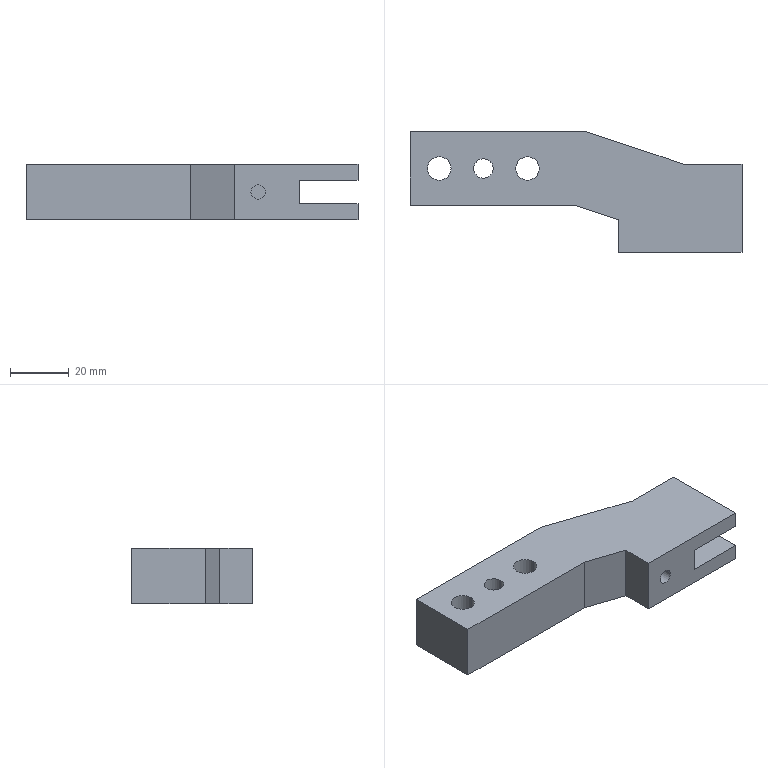Part | SolidWorks | features ICE 2, Extrusion 1 | 1 solid | 25 faces | box 113 x 41 x 19 mm | volume 51873 mm3 | plane 17 | cylinder 8 | commonest cylinder face diameters 8 x4 4.917 x2 6.647 x2
STEP:
#1=CARTESIAN_POINT('',(76.542,-1.,9.5));
#2=VERTEX_POINT('',#1);
#3=CARTESIAN_POINT('',(81.459,-1.,9.5));
#4=VERTEX_POINT('',#3);
#5=CARTESIAN_POINT('',(79.,-1.,9.5));
#6=DIRECTION('',(0.,-1.,0.));
#7=DIRECTION('',(1.,0.,0.));
#8=AXIS2_PLACEMENT_3D('',#5,#6,#7);
#9=CIRCLE('',#8,2.459);
#10=EDGE_CURVE('',#2,#4,#9,.T.);
#11=ORIENTED_EDGE('',*,*,#10,.F.);
#12=CARTESIAN_POINT('',(76.542,-16.,9.5));
#13=VERTEX_POINT('',#12);
#14=CARTESIAN_POINT('',(76.542,-1.,9.5));
#15=DIRECTION('',(0.,-1.,0.));
#16=VECTOR('',#15,1000.);
#17=LINE('',#14,#16);
#18=EDGE_CURVE('',#2,#13,#17,.T.);
#19=ORIENTED_EDGE('',*,*,#18,.T.);
#20=CARTESIAN_POINT('',(81.459,-16.,9.5));
#21=VERTEX_POINT('',#20);
#22=CARTESIAN_POINT('',(79.,-16.,9.5));
#23=DIRECTION('',(0.,-1.,0.));
#24=DIRECTION('',(1.,0.,0.));
#25=AXIS2_PLACEMENT_3D('',#22,#23,#24);
#26=CIRCLE('',#25,2.459);
#27=EDGE_CURVE('',#13,#21,#26,.T.);
#28=ORIENTED_EDGE('',*,*,#27,.T.);
#29=CARTESIAN_POINT('',(81.459,-1.,9.5));
#30=DIRECTION('',(0.,-1.,0.));
#31=VECTOR('',#30,1000.);
#32=LINE('',#29,#31);
#33=EDGE_CURVE('',#4,#21,#32,.T.);
#34=ORIENTED_EDGE('',*,*,#33,.F.);
#35=EDGE_LOOP('',(#11,#19,#28,#34));
#36=FACE_OUTER_BOUND('',#35,.T.);
#37=CARTESIAN_POINT('',(79.,-1.,9.5));
#38=DIRECTION('',(0.,-1.,0.));
#39=DIRECTION('',(1.,0.,0.));
#40=AXIS2_PLACEMENT_3D('',#37,#38,#39);
#41=CYLINDRICAL_SURFACE('',#40,2.459);
#42=ADVANCED_FACE('',(#36),#41,.F.);
#43=CARTESIAN_POINT('',(36.,12.5,19.));
#44=VERTEX_POINT('',#43);
#45=CARTESIAN_POINT('',(44.,12.5,19.));
#46=VERTEX_POINT('',#45);
#47=CARTESIAN_POINT('',(40.,12.5,19.));
#48=DIRECTION('',(0.,0.,1.));
#49=DIRECTION('',(1.,0.,0.));
#50=AXIS2_PLACEMENT_3D('',#47,#48,#49);
#51=CIRCLE('',#50,4.);
#52=EDGE_CURVE('',#44,#46,#51,.T.);
#53=ORIENTED_EDGE('',*,*,#52,.T.);
#54=CARTESIAN_POINT('',(44.,12.5,0.));
#55=VERTEX_POINT('',#54);
#56=CARTESIAN_POINT('',(44.,12.5,19.));
#57=DIRECTION('',(0.,0.,-1.));
#58=VECTOR('',#57,1000.);
#59=LINE('',#56,#58);
#60=EDGE_CURVE('',#46,#55,#59,.T.);
#61=ORIENTED_EDGE('',*,*,#60,.T.);
#62=CARTESIAN_POINT('',(36.,12.5,0.));
#63=VERTEX_POINT('',#62);
#64=CARTESIAN_POINT('',(40.,12.5,0.));
#65=DIRECTION('',(0.,0.,1.));
#66=DIRECTION('',(1.,0.,0.));
#67=AXIS2_PLACEMENT_3D('',#64,#65,#66);
#68=CIRCLE('',#67,4.);
#69=EDGE_CURVE('',#63,#55,#68,.T.);
#70=ORIENTED_EDGE('',*,*,#69,.F.);
#71=CARTESIAN_POINT('',(36.,12.5,19.));
#72=DIRECTION('',(0.,0.,-1.));
#73=VECTOR('',#72,1000.);
#74=LINE('',#71,#73);
#75=EDGE_CURVE('',#44,#63,#74,.T.);
#76=ORIENTED_EDGE('',*,*,#75,.F.);
#77=EDGE_LOOP('',(#53,#61,#70,#76));
#78=FACE_OUTER_BOUND('',#77,.T.);
#79=CARTESIAN_POINT('',(40.,12.5,19.));
#80=DIRECTION('',(0.,0.,-1.));
#81=DIRECTION('',(-1.,0.,0.));
#82=AXIS2_PLACEMENT_3D('',#79,#80,#81);
#83=CYLINDRICAL_SURFACE('',#82,4.);
#84=ADVANCED_FACE('',(#78),#83,.F.);
#85=CARTESIAN_POINT('',(21.677,12.5,19.));
#86=VERTEX_POINT('',#85);
#87=CARTESIAN_POINT('',(28.324,12.5,19.));
#88=VERTEX_POINT('',#87);
#89=CARTESIAN_POINT('',(25.,12.5,19.));
#90=DIRECTION('',(0.,0.,1.));
#91=DIRECTION('',(1.,0.,0.));
#92=AXIS2_PLACEMENT_3D('',#89,#90,#91);
#93=CIRCLE('',#92,3.324);
#94=EDGE_CURVE('',#86,#88,#93,.T.);
#95=ORIENTED_EDGE('',*,*,#94,.T.);
#96=CARTESIAN_POINT('',(28.324,12.5,0.));
#97=VERTEX_POINT('',#96);
#98=CARTESIAN_POINT('',(28.324,12.5,19.));
#99=DIRECTION('',(0.,0.,-1.));
#100=VECTOR('',#99,1000.);
#101=LINE('',#98,#100);
#102=EDGE_CURVE('',#88,#97,#101,.T.);
#103=ORIENTED_EDGE('',*,*,#102,.T.);
#104=CARTESIAN_POINT('',(21.677,12.5,0.));
#105=VERTEX_POINT('',#104);
#106=CARTESIAN_POINT('',(25.,12.5,0.));
#107=DIRECTION('',(0.,0.,1.));
#108=DIRECTION('',(1.,0.,0.));
#109=AXIS2_PLACEMENT_3D('',#106,#107,#108);
#110=CIRCLE('',#109,3.324);
#111=EDGE_CURVE('',#105,#97,#110,.T.);
#112=ORIENTED_EDGE('',*,*,#111,.F.);
#113=CARTESIAN_POINT('',(21.677,12.5,19.));
#114=DIRECTION('',(0.,0.,-1.));
#115=VECTOR('',#114,1000.);
#116=LINE('',#113,#115);
#117=EDGE_CURVE('',#86,#105,#116,.T.);
#118=ORIENTED_EDGE('',*,*,#117,.F.);
#119=EDGE_LOOP('',(#95,#103,#112,#118));
#120=FACE_OUTER_BOUND('',#119,.T.);
#121=CARTESIAN_POINT('',(25.,12.5,19.));
#122=DIRECTION('',(0.,0.,-1.));
#123=DIRECTION('',(-1.,0.,0.));
#124=AXIS2_PLACEMENT_3D('',#121,#122,#123);
#125=CYLINDRICAL_SURFACE('',#124,3.324);
#126=ADVANCED_FACE('',(#120),#125,.F.);
#127=CARTESIAN_POINT('',(6.,12.5,19.));
#128=VERTEX_POINT('',#127);
#129=CARTESIAN_POINT('',(14.,12.5,19.));
#130=VERTEX_POINT('',#129);
#131=CARTESIAN_POINT('',(10.,12.5,19.));
#132=DIRECTION('',(0.,0.,1.));
#133=DIRECTION('',(1.,0.,0.));
#134=AXIS2_PLACEMENT_3D('',#131,#132,#133);
#135=CIRCLE('',#134,4.);
#136=EDGE_CURVE('',#128,#130,#135,.T.);
#137=ORIENTED_EDGE('',*,*,#136,.T.);
#138=CARTESIAN_POINT('',(14.,12.5,0.));
#139=VERTEX_POINT('',#138);
#140=CARTESIAN_POINT('',(14.,12.5,19.));
#141=DIRECTION('',(0.,0.,-1.));
#142=VECTOR('',#141,1000.);
#143=LINE('',#140,#142);
#144=EDGE_CURVE('',#130,#139,#143,.T.);
#145=ORIENTED_EDGE('',*,*,#144,.T.);
#146=CARTESIAN_POINT('',(6.,12.5,0.));
#147=VERTEX_POINT('',#146);
#148=CARTESIAN_POINT('',(10.,12.5,0.));
#149=DIRECTION('',(0.,0.,1.));
#150=DIRECTION('',(1.,0.,0.));
#151=AXIS2_PLACEMENT_3D('',#148,#149,#150);
#152=CIRCLE('',#151,4.);
#153=EDGE_CURVE('',#147,#139,#152,.T.);
#154=ORIENTED_EDGE('',*,*,#153,.F.);
#155=CARTESIAN_POINT('',(6.,12.5,19.));
#156=DIRECTION('',(0.,0.,-1.));
#157=VECTOR('',#156,1000.);
#158=LINE('',#155,#157);
#159=EDGE_CURVE('',#128,#147,#158,.T.);
#160=ORIENTED_EDGE('',*,*,#159,.F.);
#161=EDGE_LOOP('',(#137,#145,#154,#160));
#162=FACE_OUTER_BOUND('',#161,.T.);
#163=CARTESIAN_POINT('',(10.,12.5,19.));
#164=DIRECTION('',(0.,0.,-1.));
#165=DIRECTION('',(-1.,0.,0.));
#166=AXIS2_PLACEMENT_3D('',#163,#164,#165);
#167=CYLINDRICAL_SURFACE('',#166,4.);
#168=ADVANCED_FACE('',(#162),#167,.F.);
#169=CARTESIAN_POINT('',(113.,14.,5.5));
#170=VERTEX_POINT('',#169);
#171=CARTESIAN_POINT('',(113.,14.,0.));
#172=VERTEX_POINT('',#171);
#173=CARTESIAN_POINT('',(113.,14.,19.));
#174=DIRECTION('',(0.,0.,-1.));
#175=VECTOR('',#174,1000.);
#176=LINE('',#173,#175);
#177=EDGE_CURVE('',#170,#172,#176,.T.);
#178=ORIENTED_EDGE('',*,*,#177,.F.);
#179=CARTESIAN_POINT('',(113.,-16.,5.5));
#180=VERTEX_POINT('',#179);
#181=CARTESIAN_POINT('',(113.,-16.001,5.5));
#182=DIRECTION('',(0.,1.,0.));
#183=VECTOR('',#182,1000.);
#184=LINE('',#181,#183);
#185=EDGE_CURVE('',#180,#170,#184,.T.);
#186=ORIENTED_EDGE('',*,*,#185,.F.);
#187=CARTESIAN_POINT('',(113.,-16.,0.));
#188=VERTEX_POINT('',#187);
#189=CARTESIAN_POINT('',(113.,-16.,19.));
#190=DIRECTION('',(0.,0.,-1.));
#191=VECTOR('',#190,1000.);
#192=LINE('',#189,#191);
#193=EDGE_CURVE('',#180,#188,#192,.T.);
#194=ORIENTED_EDGE('',*,*,#193,.T.);
#195=CARTESIAN_POINT('',(113.,-16.,0.));
#196=DIRECTION('',(0.,1.,0.));
#197=VECTOR('',#196,1000.);
#198=LINE('',#195,#197);
#199=EDGE_CURVE('',#188,#172,#198,.T.);
#200=ORIENTED_EDGE('',*,*,#199,.T.);
#201=EDGE_LOOP('',(#178,#186,#194,#200));
#202=FACE_OUTER_BOUND('',#201,.T.);
#203=CARTESIAN_POINT('',(113.,-16.,19.));
#204=DIRECTION('',(-1.,0.,0.));
#205=DIRECTION('',(0.,0.,1.));
#206=AXIS2_PLACEMENT_3D('',#203,#204,#205);
#207=PLANE('',#206);
#208=ADVANCED_FACE('',(#202),#207,.F.);
#209=CARTESIAN_POINT('',(93.,14.,5.5));
#210=VERTEX_POINT('',#209);
#211=CARTESIAN_POINT('',(93.,14.,0.));
#212=VERTEX_POINT('',#211);
#213=CARTESIAN_POINT('',(93.,14.,19.));
#214=DIRECTION('',(0.,0.,-1.));
#215=VECTOR('',#214,1000.);
#216=LINE('',#213,#215);
#217=EDGE_CURVE('',#210,#212,#216,.T.);
#218=ORIENTED_EDGE('',*,*,#217,.F.);
#219=CARTESIAN_POINT('',(93.,14.,5.5));
#220=DIRECTION('',(-1.,0.,0.));
#221=VECTOR('',#220,1000.);
#222=LINE('',#219,#221);
#223=EDGE_CURVE('',#170,#210,#222,.T.);
#224=ORIENTED_EDGE('',*,*,#223,.F.);
#225=ORIENTED_EDGE('',*,*,#177,.T.);
#226=CARTESIAN_POINT('',(113.,14.,0.));
#227=DIRECTION('',(-1.,0.,0.));
#228=VECTOR('',#227,1000.);
#229=LINE('',#226,#228);
#230=EDGE_CURVE('',#172,#212,#229,.T.);
#231=ORIENTED_EDGE('',*,*,#230,.T.);
#232=EDGE_LOOP('',(#218,#224,#225,#231));
#233=FACE_OUTER_BOUND('',#232,.T.);
#234=CARTESIAN_POINT('',(113.,14.,19.));
#235=DIRECTION('',(0.,-1.,0.));
#236=DIRECTION('',(1.,0.,0.));
#237=AXIS2_PLACEMENT_3D('',#234,#235,#236);
#238=PLANE('',#237);
#239=ADVANCED_FACE('',(#233),#238,.F.);
#240=ORIENTED_EDGE('',*,*,#94,.F.);
#241=CARTESIAN_POINT('',(25.,12.5,19.));
#242=DIRECTION('',(0.,0.,1.));
#243=DIRECTION('',(1.,0.,0.));
#244=AXIS2_PLACEMENT_3D('',#241,#242,#243);
#245=CIRCLE('',#244,3.324);
#246=EDGE_CURVE('',#88,#86,#245,.T.);
#247=ORIENTED_EDGE('',*,*,#246,.F.);
#248=EDGE_LOOP('',(#240,#247));
#249=FACE_BOUND('',#248,.T.);
#250=CARTESIAN_POINT('',(0.,25.,19.));
#251=VERTEX_POINT('',#250);
#252=CARTESIAN_POINT('',(0.,0.,19.));
#253=VERTEX_POINT('',#252);
#254=CARTESIAN_POINT('',(0.,25.,19.));
#255=DIRECTION('',(0.,-1.,0.));
#256=VECTOR('',#255,1000.);
#257=LINE('',#254,#256);
#258=EDGE_CURVE('',#251,#253,#257,.T.);
#259=ORIENTED_EDGE('',*,*,#258,.T.);
#260=CARTESIAN_POINT('',(56.,0.,19.));
#261=VERTEX_POINT('',#260);
#262=CARTESIAN_POINT('',(0.,0.,19.));
#263=DIRECTION('',(1.,0.,0.));
#264=VECTOR('',#263,1000.);
#265=LINE('',#262,#264);
#266=EDGE_CURVE('',#253,#261,#265,.T.);
#267=ORIENTED_EDGE('',*,*,#266,.T.);
#268=CARTESIAN_POINT('',(71.,-5.,19.));
#269=VERTEX_POINT('',#268);
#270=CARTESIAN_POINT('',(56.,0.,19.));
#271=DIRECTION('',(0.9487,-0.3162,0.));
#272=VECTOR('',#271,1000.);
#273=LINE('',#270,#272);
#274=EDGE_CURVE('',#261,#269,#273,.T.);
#275=ORIENTED_EDGE('',*,*,#274,.T.);
#276=CARTESIAN_POINT('',(71.,-16.,19.));
#277=VERTEX_POINT('',#276);
#278=CARTESIAN_POINT('',(71.,-5.,19.));
#279=DIRECTION('',(0.,-1.,0.));
#280=VECTOR('',#279,1000.);
#281=LINE('',#278,#280);
#282=EDGE_CURVE('',#269,#277,#281,.T.);
#283=ORIENTED_EDGE('',*,*,#282,.T.);
#284=CARTESIAN_POINT('',(113.,-16.,19.));
#285=VERTEX_POINT('',#284);
#286=CARTESIAN_POINT('',(71.,-16.,19.));
#287=DIRECTION('',(1.,0.,0.));
#288=VECTOR('',#287,1000.);
#289=LINE('',#286,#288);
#290=EDGE_CURVE('',#277,#285,#289,.T.);
#291=ORIENTED_EDGE('',*,*,#290,.T.);
#292=CARTESIAN_POINT('',(113.,14.,19.));
#293=VERTEX_POINT('',#292);
#294=CARTESIAN_POINT('',(113.,-16.,19.));
#295=DIRECTION('',(0.,1.,0.));
#296=VECTOR('',#295,1000.);
#297=LINE('',#294,#296);
#298=EDGE_CURVE('',#285,#293,#297,.T.);
#299=ORIENTED_EDGE('',*,*,#298,.T.);
#300=CARTESIAN_POINT('',(93.,14.,19.));
#301=VERTEX_POINT('',#300);
#302=CARTESIAN_POINT('',(113.,14.,19.));
#303=DIRECTION('',(-1.,0.,0.));
#304=VECTOR('',#303,1000.);
#305=LINE('',#302,#304);
#306=EDGE_CURVE('',#293,#301,#305,.T.);
#307=ORIENTED_EDGE('',*,*,#306,.T.);
#308=CARTESIAN_POINT('',(60.,25.,19.));
#309=VERTEX_POINT('',#308);
#310=CARTESIAN_POINT('',(93.,14.,19.));
#311=DIRECTION('',(-0.9487,0.3162,0.));
#312=VECTOR('',#311,1000.);
#313=LINE('',#310,#312);
#314=EDGE_CURVE('',#301,#309,#313,.T.);
#315=ORIENTED_EDGE('',*,*,#314,.T.);
#316=CARTESIAN_POINT('',(60.,25.,19.));
#317=DIRECTION('',(-1.,0.,0.));
#318=VECTOR('',#317,1000.);
#319=LINE('',#316,#318);
#320=EDGE_CURVE('',#309,#251,#319,.T.);
#321=ORIENTED_EDGE('',*,*,#320,.T.);
#322=EDGE_LOOP('',(#259,#267,#275,#283,#291,#299,#307,#315,#321));
#323=FACE_OUTER_BOUND('',#322,.T.);
#324=ORIENTED_EDGE('',*,*,#136,.F.);
#325=CARTESIAN_POINT('',(10.,12.5,19.));
#326=DIRECTION('',(0.,0.,1.));
#327=DIRECTION('',(1.,0.,0.));
#328=AXIS2_PLACEMENT_3D('',#325,#326,#327);
#329=CIRCLE('',#328,4.);
#330=EDGE_CURVE('',#130,#128,#329,.T.);
#331=ORIENTED_EDGE('',*,*,#330,.F.);
#332=EDGE_LOOP('',(#324,#331));
#333=FACE_BOUND('',#332,.T.);
#334=ORIENTED_EDGE('',*,*,#52,.F.);
#335=CARTESIAN_POINT('',(40.,12.5,19.));
#336=DIRECTION('',(0.,0.,1.));
#337=DIRECTION('',(1.,0.,0.));
#338=AXIS2_PLACEMENT_3D('',#335,#336,#337);
#339=CIRCLE('',#338,4.);
#340=EDGE_CURVE('',#46,#44,#339,.T.);
#341=ORIENTED_EDGE('',*,*,#340,.F.);
#342=EDGE_LOOP('',(#334,#341));
#343=FACE_BOUND('',#342,.T.);
#344=CARTESIAN_POINT('',(0.,0.,19.));
#345=DIRECTION('',(0.,0.,1.));
#346=DIRECTION('',(1.,0.,0.));
#347=AXIS2_PLACEMENT_3D('',#344,#345,#346);
#348=PLANE('',#347);
#349=ADVANCED_FACE('',(#249,#323,#333,#343),#348,.T.);
#350=CARTESIAN_POINT('',(0.,25.,0.));
#351=VERTEX_POINT('',#350);
#352=CARTESIAN_POINT('',(0.,0.,0.));
#353=VERTEX_POINT('',#352);
#354=CARTESIAN_POINT('',(0.,25.,0.));
#355=DIRECTION('',(0.,-1.,0.));
#356=VECTOR('',#355,1000.);
#357=LINE('',#354,#356);
#358=EDGE_CURVE('',#351,#353,#357,.T.);
#359=ORIENTED_EDGE('',*,*,#358,.F.);
#360=CARTESIAN_POINT('',(60.,25.,0.));
#361=VERTEX_POINT('',#360);
#362=CARTESIAN_POINT('',(60.,25.,0.));
#363=DIRECTION('',(-1.,0.,0.));
#364=VECTOR('',#363,1000.);
#365=LINE('',#362,#364);
#366=EDGE_CURVE('',#361,#351,#365,.T.);
#367=ORIENTED_EDGE('',*,*,#366,.F.);
#368=CARTESIAN_POINT('',(93.,14.,0.));
#369=DIRECTION('',(-0.9487,0.3162,0.));
#370=VECTOR('',#369,1000.);
#371=LINE('',#368,#370);
#372=EDGE_CURVE('',#212,#361,#371,.T.);
#373=ORIENTED_EDGE('',*,*,#372,.F.);
#374=ORIENTED_EDGE('',*,*,#230,.F.);
#375=ORIENTED_EDGE('',*,*,#199,.F.);
#376=CARTESIAN_POINT('',(71.,-16.,0.));
#377=VERTEX_POINT('',#376);
#378=CARTESIAN_POINT('',(71.,-16.,0.));
#379=DIRECTION('',(1.,0.,0.));
#380=VECTOR('',#379,1000.);
#381=LINE('',#378,#380);
#382=EDGE_CURVE('',#377,#188,#381,.T.);
#383=ORIENTED_EDGE('',*,*,#382,.F.);
#384=CARTESIAN_POINT('',(71.,-5.,0.));
#385=VERTEX_POINT('',#384);
#386=CARTESIAN_POINT('',(71.,-5.,0.));
#387=DIRECTION('',(0.,-1.,0.));
#388=VECTOR('',#387,1000.);
#389=LINE('',#386,#388);
#390=EDGE_CURVE('',#385,#377,#389,.T.);
#391=ORIENTED_EDGE('',*,*,#390,.F.);
#392=CARTESIAN_POINT('',(56.,0.,0.));
#393=VERTEX_POINT('',#392);
#394=CARTESIAN_POINT('',(56.,0.,0.));
#395=DIRECTION('',(0.9487,-0.3162,0.));
#396=VECTOR('',#395,1000.);
#397=LINE('',#394,#396);
#398=EDGE_CURVE('',#393,#385,#397,.T.);
#399=ORIENTED_EDGE('',*,*,#398,.F.);
#400=CARTESIAN_POINT('',(0.,0.,0.));
#401=DIRECTION('',(1.,0.,0.));
#402=VECTOR('',#401,1000.);
#403=LINE('',#400,#402);
#404=EDGE_CURVE('',#353,#393,#403,.T.);
#405=ORIENTED_EDGE('',*,*,#404,.F.);
#406=EDGE_LOOP('',(#359,#367,#373,#374,#375,#383,#391,#399,#405));
#407=FACE_OUTER_BOUND('',#406,.T.);
#408=ORIENTED_EDGE('',*,*,#153,.T.);
#409=CARTESIAN_POINT('',(10.,12.5,0.));
#410=DIRECTION('',(0.,0.,1.));
#411=DIRECTION('',(1.,0.,0.));
#412=AXIS2_PLACEMENT_3D('',#409,#410,#411);
#413=CIRCLE('',#412,4.);
#414=EDGE_CURVE('',#139,#147,#413,.T.);
#415=ORIENTED_EDGE('',*,*,#414,.T.);
#416=EDGE_LOOP('',(#408,#415));
#417=FACE_BOUND('',#416,.T.);
#418=ORIENTED_EDGE('',*,*,#111,.T.);
#419=CARTESIAN_POINT('',(25.,12.5,0.));
#420=DIRECTION('',(0.,0.,1.));
#421=DIRECTION('',(1.,0.,0.));
#422=AXIS2_PLACEMENT_3D('',#419,#420,#421);
#423=CIRCLE('',#422,3.324);
#424=EDGE_CURVE('',#97,#105,#423,.T.);
#425=ORIENTED_EDGE('',*,*,#424,.T.);
#426=EDGE_LOOP('',(#418,#425));
#427=FACE_BOUND('',#426,.T.);
#428=ORIENTED_EDGE('',*,*,#69,.T.);
#429=CARTESIAN_POINT('',(40.,12.5,0.));
#430=DIRECTION('',(0.,0.,1.));
#431=DIRECTION('',(1.,0.,0.));
#432=AXIS2_PLACEMENT_3D('',#429,#430,#431);
#433=CIRCLE('',#432,4.);
#434=EDGE_CURVE('',#55,#63,#433,.T.);
#435=ORIENTED_EDGE('',*,*,#434,.T.);
#436=EDGE_LOOP('',(#428,#435));
#437=FACE_BOUND('',#436,.T.);
#438=CARTESIAN_POINT('',(0.,0.,0.));
#439=DIRECTION('',(0.,0.,1.));
#440=DIRECTION('',(1.,0.,0.));
#441=AXIS2_PLACEMENT_3D('',#438,#439,#440);
#442=PLANE('',#441);
#443=ADVANCED_FACE('',(#407,#417,#427,#437),#442,.F.);
#444=ORIENTED_EDGE('',*,*,#358,.T.);
#445=CARTESIAN_POINT('',(0.,0.,19.));
#446=DIRECTION('',(0.,0.,-1.));
#447=VECTOR('',#446,1000.);
#448=LINE('',#445,#447);
#449=EDGE_CURVE('',#253,#353,#448,.T.);
#450=ORIENTED_EDGE('',*,*,#449,.F.);
#451=ORIENTED_EDGE('',*,*,#258,.F.);
#452=CARTESIAN_POINT('',(0.,25.,19.));
#453=DIRECTION('',(0.,0.,-1.));
#454=VECTOR('',#453,1000.);
#455=LINE('',#452,#454);
#456=EDGE_CURVE('',#251,#351,#455,.T.);
#457=ORIENTED_EDGE('',*,*,#456,.T.);
#458=EDGE_LOOP('',(#444,#450,#451,#457));
#459=FACE_OUTER_BOUND('',#458,.T.);
#460=CARTESIAN_POINT('',(0.,25.,19.));
#461=DIRECTION('',(1.,0.,0.));
#462=DIRECTION('',(0.,0.,-1.));
#463=AXIS2_PLACEMENT_3D('',#460,#461,#462);
#464=PLANE('',#463);
#465=ADVANCED_FACE('',(#459),#464,.F.);
#466=ORIENTED_EDGE('',*,*,#404,.T.);
#467=CARTESIAN_POINT('',(56.,0.,19.));
#468=DIRECTION('',(0.,0.,-1.));
#469=VECTOR('',#468,1000.);
#470=LINE('',#467,#469);
#471=EDGE_CURVE('',#261,#393,#470,.T.);
#472=ORIENTED_EDGE('',*,*,#471,.F.);
#473=ORIENTED_EDGE('',*,*,#266,.F.);
#474=ORIENTED_EDGE('',*,*,#449,.T.);
#475=EDGE_LOOP('',(#466,#472,#473,#474));
#476=FACE_OUTER_BOUND('',#475,.T.);
#477=CARTESIAN_POINT('',(0.,0.,19.));
#478=DIRECTION('',(0.,1.,0.));
#479=DIRECTION('',(0.,0.,1.));
#480=AXIS2_PLACEMENT_3D('',#477,#478,#479);
#481=PLANE('',#480);
#482=ADVANCED_FACE('',(#476),#481,.F.);
#483=ORIENTED_EDGE('',*,*,#398,.T.);
#484=CARTESIAN_POINT('',(71.,-5.,19.));
#485=DIRECTION('',(0.,0.,-1.));
#486=VECTOR('',#485,1000.);
#487=LINE('',#484,#486);
#488=EDGE_CURVE('',#269,#385,#487,.T.);
#489=ORIENTED_EDGE('',*,*,#488,.F.);
#490=ORIENTED_EDGE('',*,*,#274,.F.);
#491=ORIENTED_EDGE('',*,*,#471,.T.);
#492=EDGE_LOOP('',(#483,#489,#490,#491));
#493=FACE_OUTER_BOUND('',#492,.T.);
#494=CARTESIAN_POINT('',(56.,0.,19.));
#495=DIRECTION('',(0.3162,0.9487,0.));
#496=DIRECTION('',(-0.9487,0.3162,0.));
#497=AXIS2_PLACEMENT_3D('',#494,#495,#496);
#498=PLANE('',#497);
#499=ADVANCED_FACE('',(#493),#498,.F.);
#500=ORIENTED_EDGE('',*,*,#390,.T.);
#501=CARTESIAN_POINT('',(71.,-16.,19.));
#502=DIRECTION('',(0.,0.,-1.));
#503=VECTOR('',#502,1000.);
#504=LINE('',#501,#503);
#505=EDGE_CURVE('',#277,#377,#504,.T.);
#506=ORIENTED_EDGE('',*,*,#505,.F.);
#507=ORIENTED_EDGE('',*,*,#282,.F.);
#508=ORIENTED_EDGE('',*,*,#488,.T.);
#509=EDGE_LOOP('',(#500,#506,#507,#508));
#510=FACE_OUTER_BOUND('',#509,.T.);
#511=CARTESIAN_POINT('',(71.,-5.,19.));
#512=DIRECTION('',(1.,0.,0.));
#513=DIRECTION('',(0.,1.,0.));
#514=AXIS2_PLACEMENT_3D('',#511,#512,#513);
#515=PLANE('',#514);
#516=ADVANCED_FACE('',(#510),#515,.F.);
#517=CARTESIAN_POINT('',(79.,-16.,9.5));
#518=DIRECTION('',(0.,-1.,0.));
#519=DIRECTION('',(1.,0.,0.));
#520=AXIS2_PLACEMENT_3D('',#517,#518,#519);
#521=CIRCLE('',#520,2.459);
#522=EDGE_CURVE('',#21,#13,#521,.T.);
#523=ORIENTED_EDGE('',*,*,#522,.F.);
#524=ORIENTED_EDGE('',*,*,#27,.F.);
#525=EDGE_LOOP('',(#523,#524));
#526=FACE_BOUND('',#525,.T.);
#527=ORIENTED_EDGE('',*,*,#193,.F.);
#528=CARTESIAN_POINT('',(93.,-16.,5.5));
#529=VERTEX_POINT('',#528);
#530=CARTESIAN_POINT('',(93.,-16.,5.5));
#531=DIRECTION('',(1.,0.,0.));
#532=VECTOR('',#531,1000.);
#533=LINE('',#530,#532);
#534=EDGE_CURVE('',#529,#180,#533,.T.);
#535=ORIENTED_EDGE('',*,*,#534,.F.);
#536=CARTESIAN_POINT('',(93.,-16.,13.5));
#537=VERTEX_POINT('',#536);
#538=CARTESIAN_POINT('',(93.,-16.,5.5));
#539=DIRECTION('',(0.,0.,-1.));
#540=VECTOR('',#539,1000.);
#541=LINE('',#538,#540);
#542=EDGE_CURVE('',#537,#529,#541,.T.);
#543=ORIENTED_EDGE('',*,*,#542,.F.);
#544=CARTESIAN_POINT('',(113.,-16.,13.5));
#545=VERTEX_POINT('',#544);
#546=CARTESIAN_POINT('',(93.,-16.,13.5));
#547=DIRECTION('',(-1.,0.,0.));
#548=VECTOR('',#547,1000.);
#549=LINE('',#546,#548);
#550=EDGE_CURVE('',#545,#537,#549,.T.);
#551=ORIENTED_EDGE('',*,*,#550,.F.);
#552=CARTESIAN_POINT('',(113.,-16.,19.));
#553=DIRECTION('',(0.,0.,-1.));
#554=VECTOR('',#553,1000.);
#555=LINE('',#552,#554);
#556=EDGE_CURVE('',#285,#545,#555,.T.);
#557=ORIENTED_EDGE('',*,*,#556,.F.);
#558=ORIENTED_EDGE('',*,*,#290,.F.);
#559=ORIENTED_EDGE('',*,*,#505,.T.);
#560=ORIENTED_EDGE('',*,*,#382,.T.);
#561=EDGE_LOOP('',(#527,#535,#543,#551,#557,#558,#559,#560));
#562=FACE_OUTER_BOUND('',#561,.T.);
#563=CARTESIAN_POINT('',(71.,-16.,19.));
#564=DIRECTION('',(0.,1.,0.));
#565=DIRECTION('',(-1.,0.,0.));
#566=AXIS2_PLACEMENT_3D('',#563,#564,#565);
#567=PLANE('',#566);
#568=ADVANCED_FACE('',(#526,#562),#567,.F.);
#569=ORIENTED_EDGE('',*,*,#556,.T.);
#570=CARTESIAN_POINT('',(113.,14.,13.5));
#571=VERTEX_POINT('',#570);
#572=CARTESIAN_POINT('',(113.,-16.001,13.5));
#573=DIRECTION('',(0.,1.,0.));
#574=VECTOR('',#573,1000.);
#575=LINE('',#572,#574);
#576=EDGE_CURVE('',#545,#571,#575,.T.);
#577=ORIENTED_EDGE('',*,*,#576,.T.);
#578=CARTESIAN_POINT('',(113.,14.,19.));
#579=DIRECTION('',(0.,0.,-1.));
#580=VECTOR('',#579,1000.);
#581=LINE('',#578,#580);
#582=EDGE_CURVE('',#293,#571,#581,.T.);
#583=ORIENTED_EDGE('',*,*,#582,.F.);
#584=ORIENTED_EDGE('',*,*,#298,.F.);
#585=EDGE_LOOP('',(#569,#577,#583,#584));
#586=FACE_OUTER_BOUND('',#585,.T.);
#587=CARTESIAN_POINT('',(113.,-16.,19.));
#588=DIRECTION('',(-1.,0.,0.));
#589=DIRECTION('',(0.,0.,1.));
#590=AXIS2_PLACEMENT_3D('',#587,#588,#589);
#591=PLANE('',#590);
#592=ADVANCED_FACE('',(#586),#591,.F.);
#593=ORIENTED_EDGE('',*,*,#582,.T.);
#594=CARTESIAN_POINT('',(93.,14.,13.5));
#595=VERTEX_POINT('',#594);
#596=CARTESIAN_POINT('',(93.,14.,13.5));
#597=DIRECTION('',(1.,0.,0.));
#598=VECTOR('',#597,1000.);
#599=LINE('',#596,#598);
#600=EDGE_CURVE('',#595,#571,#599,.T.);
#601=ORIENTED_EDGE('',*,*,#600,.F.);
#602=CARTESIAN_POINT('',(93.,14.,19.));
#603=DIRECTION('',(0.,0.,-1.));
#604=VECTOR('',#603,1000.);
#605=LINE('',#602,#604);
#606=EDGE_CURVE('',#301,#595,#605,.T.);
#607=ORIENTED_EDGE('',*,*,#606,.F.);
#608=ORIENTED_EDGE('',*,*,#306,.F.);
#609=EDGE_LOOP('',(#593,#601,#607,#608));
#610=FACE_OUTER_BOUND('',#609,.T.);
#611=CARTESIAN_POINT('',(113.,14.,19.));
#612=DIRECTION('',(0.,-1.,0.));
#613=DIRECTION('',(1.,0.,0.));
#614=AXIS2_PLACEMENT_3D('',#611,#612,#613);
#615=PLANE('',#614);
#616=ADVANCED_FACE('',(#610),#615,.F.);
#617=ORIENTED_EDGE('',*,*,#372,.T.);
#618=CARTESIAN_POINT('',(60.,25.,19.));
#619=DIRECTION('',(0.,0.,-1.));
#620=VECTOR('',#619,1000.);
#621=LINE('',#618,#620);
#622=EDGE_CURVE('',#309,#361,#621,.T.);
#623=ORIENTED_EDGE('',*,*,#622,.F.);
#624=ORIENTED_EDGE('',*,*,#314,.F.);
#625=ORIENTED_EDGE('',*,*,#606,.T.);
#626=CARTESIAN_POINT('',(93.,14.,5.5));
#627=DIRECTION('',(0.,0.,1.));
#628=VECTOR('',#627,1000.);
#629=LINE('',#626,#628);
#630=EDGE_CURVE('',#210,#595,#629,.T.);
#631=ORIENTED_EDGE('',*,*,#630,.F.);
#632=ORIENTED_EDGE('',*,*,#217,.T.);
#633=EDGE_LOOP('',(#617,#623,#624,#625,#631,#632));
#634=FACE_OUTER_BOUND('',#633,.T.);
#635=CARTESIAN_POINT('',(93.,14.,19.));
#636=DIRECTION('',(-0.3162,-0.9487,0.));
#637=DIRECTION('',(0.9487,-0.3162,0.));
#638=AXIS2_PLACEMENT_3D('',#635,#636,#637);
#639=PLANE('',#638);
#640=ADVANCED_FACE('',(#634),#639,.F.);
#641=ORIENTED_EDGE('',*,*,#366,.T.);
#642=ORIENTED_EDGE('',*,*,#456,.F.);
#643=ORIENTED_EDGE('',*,*,#320,.F.);
#644=ORIENTED_EDGE('',*,*,#622,.T.);
#645=EDGE_LOOP('',(#641,#642,#643,#644));
#646=FACE_OUTER_BOUND('',#645,.T.);
#647=CARTESIAN_POINT('',(60.,25.,19.));
#648=DIRECTION('',(0.,-1.,0.));
#649=DIRECTION('',(1.,0.,0.));
#650=AXIS2_PLACEMENT_3D('',#647,#648,#649);
#651=PLANE('',#650);
#652=ADVANCED_FACE('',(#646),#651,.F.);
#653=ORIENTED_EDGE('',*,*,#144,.F.);
#654=ORIENTED_EDGE('',*,*,#330,.T.);
#655=ORIENTED_EDGE('',*,*,#159,.T.);
#656=ORIENTED_EDGE('',*,*,#414,.F.);
#657=EDGE_LOOP('',(#653,#654,#655,#656));
#658=FACE_OUTER_BOUND('',#657,.T.);
#659=CARTESIAN_POINT('',(10.,12.5,19.));
#660=DIRECTION('',(0.,0.,-1.));
#661=DIRECTION('',(-1.,0.,0.));
#662=AXIS2_PLACEMENT_3D('',#659,#660,#661);
#663=CYLINDRICAL_SURFACE('',#662,4.);
#664=ADVANCED_FACE('',(#658),#663,.F.);
#665=ORIENTED_EDGE('',*,*,#102,.F.);
#666=ORIENTED_EDGE('',*,*,#246,.T.);
#667=ORIENTED_EDGE('',*,*,#117,.T.);
#668=ORIENTED_EDGE('',*,*,#424,.F.);
#669=EDGE_LOOP('',(#665,#666,#667,#668));
#670=FACE_OUTER_BOUND('',#669,.T.);
#671=CARTESIAN_POINT('',(25.,12.5,19.));
#672=DIRECTION('',(0.,0.,-1.));
#673=DIRECTION('',(-1.,0.,0.));
#674=AXIS2_PLACEMENT_3D('',#671,#672,#673);
#675=CYLINDRICAL_SURFACE('',#674,3.324);
#676=ADVANCED_FACE('',(#670),#675,.F.);
#677=ORIENTED_EDGE('',*,*,#60,.F.);
#678=ORIENTED_EDGE('',*,*,#340,.T.);
#679=ORIENTED_EDGE('',*,*,#75,.T.);
#680=ORIENTED_EDGE('',*,*,#434,.F.);
#681=EDGE_LOOP('',(#677,#678,#679,#680));
#682=FACE_OUTER_BOUND('',#681,.T.);
#683=CARTESIAN_POINT('',(40.,12.5,19.));
#684=DIRECTION('',(0.,0.,-1.));
#685=DIRECTION('',(-1.,0.,0.));
#686=AXIS2_PLACEMENT_3D('',#683,#684,#685);
#687=CYLINDRICAL_SURFACE('',#686,4.);
#688=ADVANCED_FACE('',(#682),#687,.F.);
#689=ORIENTED_EDGE('',*,*,#542,.T.);
#690=CARTESIAN_POINT('',(93.,-16.001,5.5));
#691=DIRECTION('',(0.,1.,0.));
#692=VECTOR('',#691,1000.);
#693=LINE('',#690,#692);
#694=EDGE_CURVE('',#529,#210,#693,.T.);
#695=ORIENTED_EDGE('',*,*,#694,.T.);
#696=ORIENTED_EDGE('',*,*,#630,.T.);
#697=CARTESIAN_POINT('',(93.,-16.001,13.5));
#698=DIRECTION('',(0.,1.,0.));
#699=VECTOR('',#698,1000.);
#700=LINE('',#697,#699);
#701=EDGE_CURVE('',#537,#595,#700,.T.);
#702=ORIENTED_EDGE('',*,*,#701,.F.);
#703=EDGE_LOOP('',(#689,#695,#696,#702));
#704=FACE_OUTER_BOUND('',#703,.T.);
#705=CARTESIAN_POINT('',(93.,-16.001,5.5));
#706=DIRECTION('',(-1.,0.,0.));
#707=DIRECTION('',(0.,-1.,0.));
#708=AXIS2_PLACEMENT_3D('',#705,#706,#707);
#709=PLANE('',#708);
#710=ADVANCED_FACE('',(#704),#709,.F.);
#711=ORIENTED_EDGE('',*,*,#534,.T.);
#712=ORIENTED_EDGE('',*,*,#185,.T.);
#713=ORIENTED_EDGE('',*,*,#223,.T.);
#714=ORIENTED_EDGE('',*,*,#694,.F.);
#715=EDGE_LOOP('',(#711,#712,#713,#714));
#716=FACE_OUTER_BOUND('',#715,.T.);
#717=CARTESIAN_POINT('',(93.,-16.001,5.5));
#718=DIRECTION('',(0.,0.,-1.));
#719=DIRECTION('',(-1.,0.,0.));
#720=AXIS2_PLACEMENT_3D('',#717,#718,#719);
#721=PLANE('',#720);
#722=ADVANCED_FACE('',(#716),#721,.F.);
#723=ORIENTED_EDGE('',*,*,#550,.T.);
#724=ORIENTED_EDGE('',*,*,#701,.T.);
#725=ORIENTED_EDGE('',*,*,#600,.T.);
#726=ORIENTED_EDGE('',*,*,#576,.F.);
#727=EDGE_LOOP('',(#723,#724,#725,#726));
#728=FACE_OUTER_BOUND('',#727,.T.);
#729=CARTESIAN_POINT('',(93.,-16.001,13.5));
#730=DIRECTION('',(0.,0.,1.));
#731=DIRECTION('',(1.,0.,0.));
#732=AXIS2_PLACEMENT_3D('',#729,#730,#731);
#733=PLANE('',#732);
#734=ADVANCED_FACE('',(#728),#733,.F.);
#735=ORIENTED_EDGE('',*,*,#18,.F.);
#736=CARTESIAN_POINT('',(79.,-1.,9.5));
#737=DIRECTION('',(0.,-1.,0.));
#738=DIRECTION('',(1.,0.,0.));
#739=AXIS2_PLACEMENT_3D('',#736,#737,#738);
#740=CIRCLE('',#739,2.459);
#741=EDGE_CURVE('',#4,#2,#740,.T.);
#742=ORIENTED_EDGE('',*,*,#741,.F.);
#743=ORIENTED_EDGE('',*,*,#33,.T.);
#744=ORIENTED_EDGE('',*,*,#522,.T.);
#745=EDGE_LOOP('',(#735,#742,#743,#744));
#746=FACE_OUTER_BOUND('',#745,.T.);
#747=CARTESIAN_POINT('',(79.,-1.,9.5));
#748=DIRECTION('',(0.,-1.,0.));
#749=DIRECTION('',(1.,0.,0.));
#750=AXIS2_PLACEMENT_3D('',#747,#748,#749);
#751=CYLINDRICAL_SURFACE('',#750,2.459);
#752=ADVANCED_FACE('',(#746),#751,.F.);
#753=ORIENTED_EDGE('',*,*,#741,.T.);
#754=ORIENTED_EDGE('',*,*,#10,.T.);
#755=EDGE_LOOP('',(#753,#754));
#756=FACE_OUTER_BOUND('',#755,.T.);
#757=CARTESIAN_POINT('',(79.,-1.,9.5));
#758=DIRECTION('',(0.,-1.,0.));
#759=DIRECTION('',(1.,0.,0.));
#760=AXIS2_PLACEMENT_3D('',#757,#758,#759);
#761=PLANE('',#760);
#762=ADVANCED_FACE('',(#756),#761,.T.);
#763=CLOSED_SHELL('',(#42,#84,#126,#168,#208,#239,#349,#443,#465,#482,#499,#516,#568,#592,#616,#640,#652,#664,#676,#688,#710,#722,#734,#752,#762));
#764=MANIFOLD_SOLID_BREP('',#763);
#765=CARTESIAN_POINT('',(0.,0.,0.));
#766=DIRECTION('',(0.,0.,1.));
#767=DIRECTION('',(1.,0.,0.));
#768=AXIS2_PLACEMENT_3D('',#765,#766,#767);
#769=(LENGTH_UNIT()NAMED_UNIT(*)SI_UNIT(.MILLI.,.METRE.));
#770=UNCERTAINTY_MEASURE_WITH_UNIT(LENGTH_MEASURE(0.00001),#769,'','');
#771=(NAMED_UNIT(*)PLANE_ANGLE_UNIT()SI_UNIT($,.RADIAN.));
#772=(NAMED_UNIT(*)SI_UNIT($,.STERADIAN.)SOLID_ANGLE_UNIT());
#773=(GEOMETRIC_REPRESENTATION_CONTEXT(3)GLOBAL_UNCERTAINTY_ASSIGNED_CONTEXT((#770))GLOBAL_UNIT_ASSIGNED_CONTEXT((#769,#771,#772))REPRESENTATION_CONTEXT('',''));
#774=ADVANCED_BREP_SHAPE_REPRESENTATION('',(#764,#768),#773);